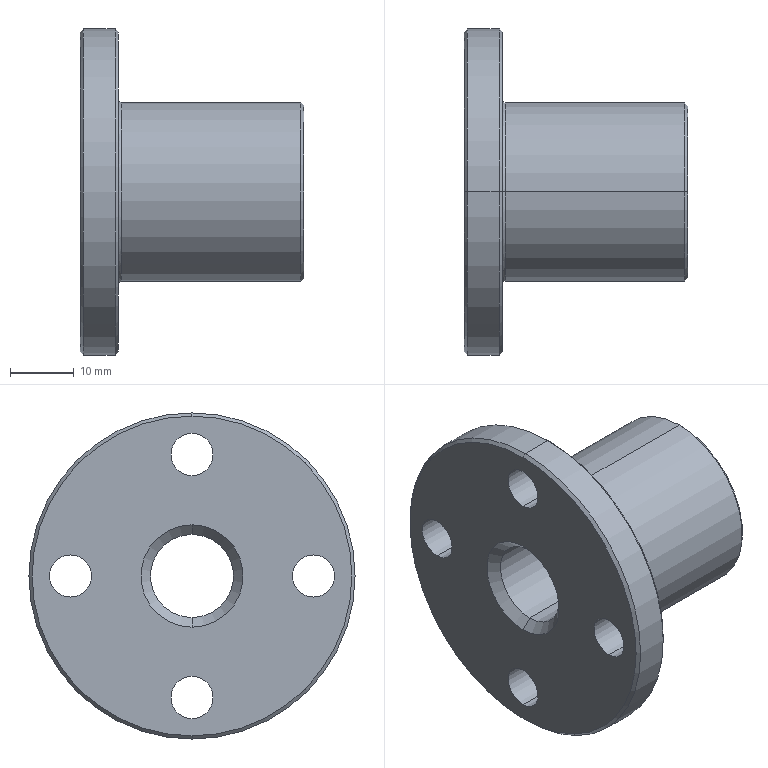Part | STEP file | 0230_003_MTSFR16 | 1 solid | 29 faces | box 35 x 51 x 51 mm | volume 24500 mm3 | cylinder 14 | cone 10 | plane 3 | spline 2 | commonest cylinder face diameters 6.6 x8 13 x2 28 x2 51 x2